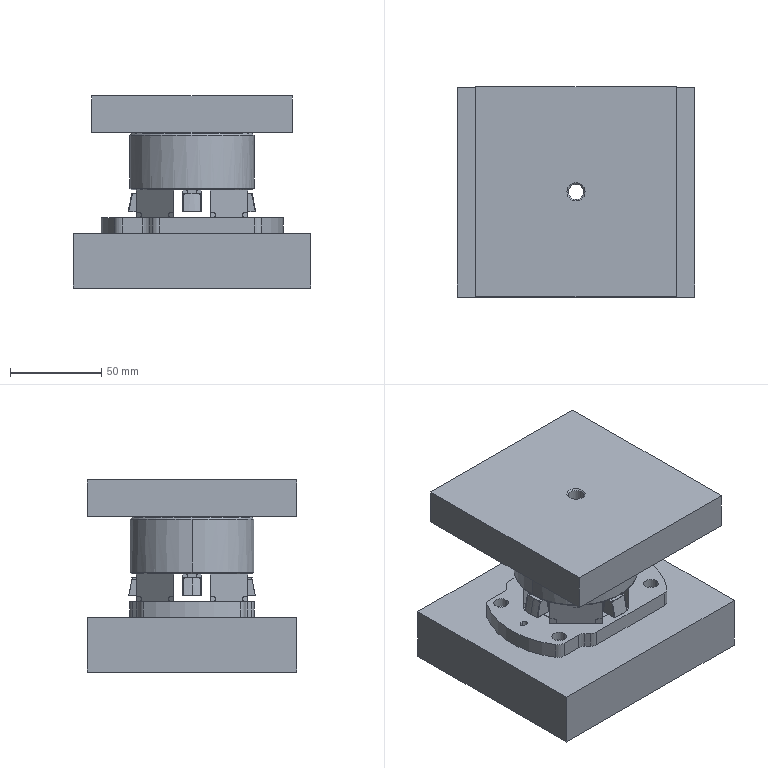NC program | NX | posted with a generic post | part box 130 x 115 x 105.2 mm
Lines 1 to 45 of 3709:
N10 G17 G21 G94 G90
(DRILLING , TOOL : Φ10_CHAMFER)
N12 T02 M6
N14 G54
N16 G17 G0 G90 X35.5 Y22.5 B0. C0. S2000 M3
N18 G43 Z65.2 H2
N20 G94 G83 G98 Z4.3 F150. Q2. R22.5
N22 Y-22.5
N24 X-35.5
N26 Y22.5
N28 G80
N30 G0 X-35.5 Y22.5 Z65.2
N32 M5
(110 , TOOL : DRILL_D4.5)
N34 T09 M6
N36 G54
N38 G17 G0 G90 X35.5 Y-22.5 B0. C0. S2000 M3
N40 G43 Z105.2 H9
N42 G94 G82 G98 Z-1.799 F100. P200 R9.5
N44 Y22.5
N46 X-35.5
N48 Y-22.5
N50 G80
N52 G0 X-35.5 Y-22.5 Z105.2
N54 M5
(111 , TOOL : D8-55_PLUNGE)
N56 T10 M6
N58 G54
N60 G17 G0 G90 X35.5 Y-22.5 B0. C0. S1600 M3
N62 G43 Z105.2 H10
N64 G94 G82 G98 Z3.5 F200. P200 R9.5
N66 Y22.5
N68 X-35.5
N70 Y-22.5
N72 G80
N74 G0 X-35.5 Y-22.5 Z105.2
N76 M5